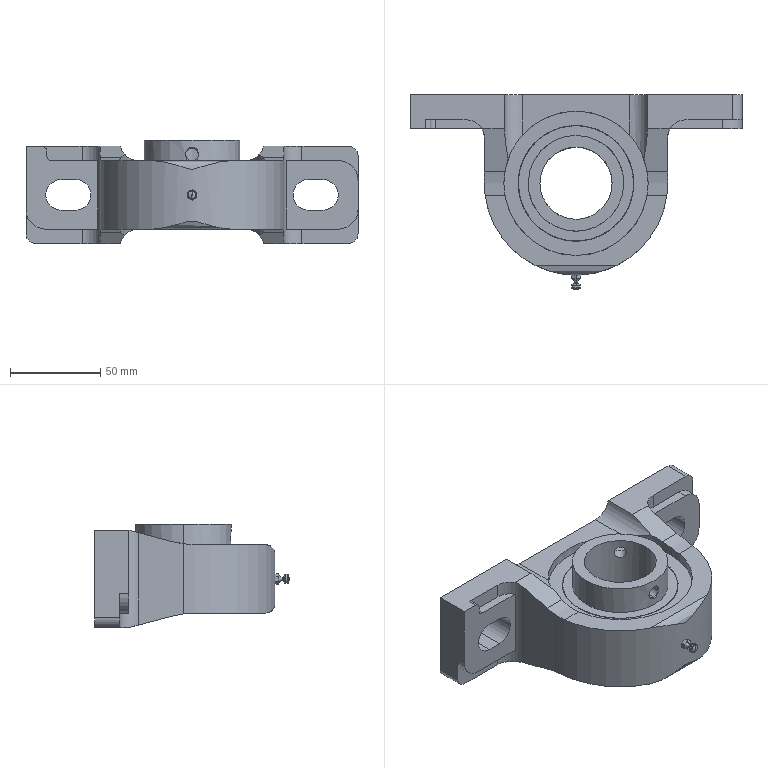Part | SolidWorks | features BaseBody 1 | 1 solid | 109 faces | box 184 x 108 x 57.2 mm | volume 359196 mm3 | plane 46 | cylinder 43 | spline 12 | cone 6 | torus 2 | commonest cylinder face diameters 20.32 x6 101.6 x5 6.917 x4 17 x4 53 x4 80 x4